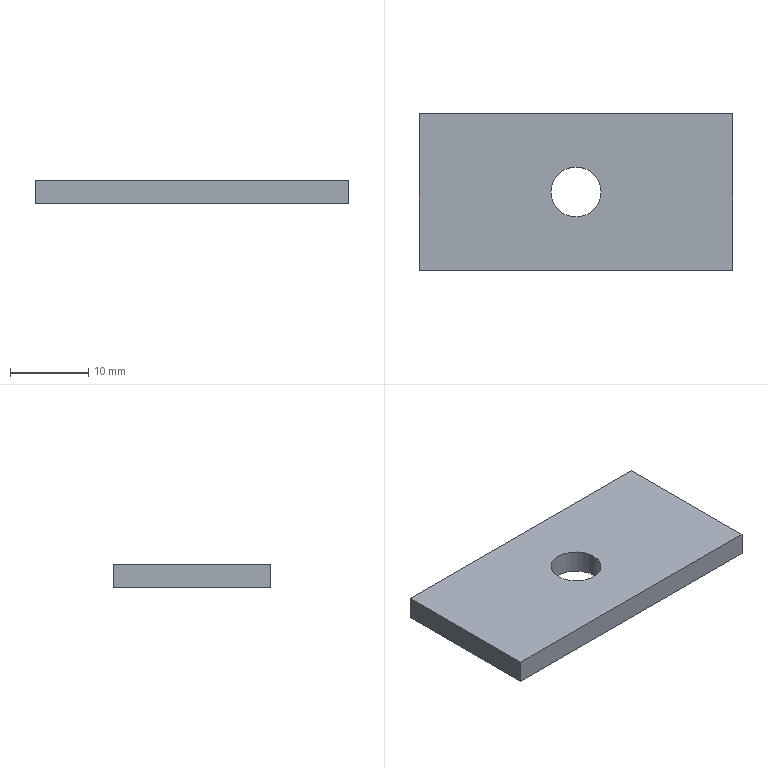Part | SolidWorks | features Extrusion 1, ICE 1 | 1 solid | 8 faces | box 40 x 20 x 3 mm | volume 2303 mm3 | plane 6 | cylinder 2 | commonest cylinder face diameters 6.4 x2
STEP:
#1=CARTESIAN_POINT('',(-3.2,0.,-1.5));
#2=VERTEX_POINT('',#1);
#3=CARTESIAN_POINT('',(3.2,0.,-1.5));
#4=VERTEX_POINT('',#3);
#5=CARTESIAN_POINT('',(0.,0.,-1.5));
#6=DIRECTION('',(0.,0.,1.));
#7=DIRECTION('',(1.,0.,0.));
#8=AXIS2_PLACEMENT_3D('',#5,#6,#7);
#9=CIRCLE('',#8,3.2);
#10=EDGE_CURVE('',#2,#4,#9,.T.);
#11=ORIENTED_EDGE('',*,*,#10,.F.);
#12=CARTESIAN_POINT('',(-3.2,0.,1.5));
#13=VERTEX_POINT('',#12);
#14=CARTESIAN_POINT('',(-3.2,0.,-11.5));
#15=DIRECTION('',(0.,0.,1.));
#16=VECTOR('',#15,1000.);
#17=LINE('',#14,#16);
#18=EDGE_CURVE('',#2,#13,#17,.T.);
#19=ORIENTED_EDGE('',*,*,#18,.T.);
#20=CARTESIAN_POINT('',(3.2,0.,1.5));
#21=VERTEX_POINT('',#20);
#22=CARTESIAN_POINT('',(0.,0.,1.5));
#23=DIRECTION('',(0.,0.,1.));
#24=DIRECTION('',(1.,0.,0.));
#25=AXIS2_PLACEMENT_3D('',#22,#23,#24);
#26=CIRCLE('',#25,3.2);
#27=EDGE_CURVE('',#13,#21,#26,.T.);
#28=ORIENTED_EDGE('',*,*,#27,.T.);
#29=CARTESIAN_POINT('',(3.2,0.,-11.5));
#30=DIRECTION('',(0.,0.,1.));
#31=VECTOR('',#30,1000.);
#32=LINE('',#29,#31);
#33=EDGE_CURVE('',#4,#21,#32,.T.);
#34=ORIENTED_EDGE('',*,*,#33,.F.);
#35=EDGE_LOOP('',(#11,#19,#28,#34));
#36=FACE_OUTER_BOUND('',#35,.T.);
#37=CARTESIAN_POINT('',(0.,0.,-11.5));
#38=DIRECTION('',(0.,0.,1.));
#39=DIRECTION('',(1.,0.,0.));
#40=AXIS2_PLACEMENT_3D('',#37,#38,#39);
#41=CYLINDRICAL_SURFACE('',#40,3.2);
#42=ADVANCED_FACE('',(#36),#41,.F.);
#43=CARTESIAN_POINT('',(-20.,10.,1.5));
#44=VERTEX_POINT('',#43);
#45=CARTESIAN_POINT('',(-20.,-10.,1.5));
#46=VERTEX_POINT('',#45);
#47=CARTESIAN_POINT('',(-20.,10.,1.5));
#48=DIRECTION('',(0.,-1.,0.));
#49=VECTOR('',#48,1000.);
#50=LINE('',#47,#49);
#51=EDGE_CURVE('',#44,#46,#50,.T.);
#52=ORIENTED_EDGE('',*,*,#51,.F.);
#53=CARTESIAN_POINT('',(-20.,10.,-1.5));
#54=VERTEX_POINT('',#53);
#55=CARTESIAN_POINT('',(-20.,10.,-1.5));
#56=DIRECTION('',(0.,0.,1.));
#57=VECTOR('',#56,1000.);
#58=LINE('',#55,#57);
#59=EDGE_CURVE('',#54,#44,#58,.T.);
#60=ORIENTED_EDGE('',*,*,#59,.F.);
#61=CARTESIAN_POINT('',(-20.,-10.,-1.5));
#62=VERTEX_POINT('',#61);
#63=CARTESIAN_POINT('',(-20.,10.,-1.5));
#64=DIRECTION('',(0.,-1.,0.));
#65=VECTOR('',#64,1000.);
#66=LINE('',#63,#65);
#67=EDGE_CURVE('',#54,#62,#66,.T.);
#68=ORIENTED_EDGE('',*,*,#67,.T.);
#69=CARTESIAN_POINT('',(-20.,-10.,-1.5));
#70=DIRECTION('',(0.,0.,1.));
#71=VECTOR('',#70,1000.);
#72=LINE('',#69,#71);
#73=EDGE_CURVE('',#62,#46,#72,.T.);
#74=ORIENTED_EDGE('',*,*,#73,.T.);
#75=EDGE_LOOP('',(#52,#60,#68,#74));
#76=FACE_OUTER_BOUND('',#75,.T.);
#77=CARTESIAN_POINT('',(-20.,10.,-1.5));
#78=DIRECTION('',(-1.,0.,0.));
#79=DIRECTION('',(0.,0.,1.));
#80=AXIS2_PLACEMENT_3D('',#77,#78,#79);
#81=PLANE('',#80);
#82=ADVANCED_FACE('',(#76),#81,.T.);
#83=CARTESIAN_POINT('',(20.,10.,1.5));
#84=VERTEX_POINT('',#83);
#85=CARTESIAN_POINT('',(20.,10.,1.5));
#86=DIRECTION('',(-1.,0.,0.));
#87=VECTOR('',#86,1000.);
#88=LINE('',#85,#87);
#89=EDGE_CURVE('',#84,#44,#88,.T.);
#90=ORIENTED_EDGE('',*,*,#89,.F.);
#91=CARTESIAN_POINT('',(20.,10.,-1.5));
#92=VERTEX_POINT('',#91);
#93=CARTESIAN_POINT('',(20.,10.,-1.5));
#94=DIRECTION('',(0.,0.,1.));
#95=VECTOR('',#94,1000.);
#96=LINE('',#93,#95);
#97=EDGE_CURVE('',#92,#84,#96,.T.);
#98=ORIENTED_EDGE('',*,*,#97,.F.);
#99=CARTESIAN_POINT('',(20.,10.,-1.5));
#100=DIRECTION('',(-1.,0.,0.));
#101=VECTOR('',#100,1000.);
#102=LINE('',#99,#101);
#103=EDGE_CURVE('',#92,#54,#102,.T.);
#104=ORIENTED_EDGE('',*,*,#103,.T.);
#105=ORIENTED_EDGE('',*,*,#59,.T.);
#106=EDGE_LOOP('',(#90,#98,#104,#105));
#107=FACE_OUTER_BOUND('',#106,.T.);
#108=CARTESIAN_POINT('',(20.,10.,-1.5));
#109=DIRECTION('',(0.,1.,0.));
#110=DIRECTION('',(0.,0.,1.));
#111=AXIS2_PLACEMENT_3D('',#108,#109,#110);
#112=PLANE('',#111);
#113=ADVANCED_FACE('',(#107),#112,.T.);
#114=CARTESIAN_POINT('',(20.,-10.,1.5));
#115=VERTEX_POINT('',#114);
#116=CARTESIAN_POINT('',(20.,-10.,1.5));
#117=DIRECTION('',(0.,1.,0.));
#118=VECTOR('',#117,1000.);
#119=LINE('',#116,#118);
#120=EDGE_CURVE('',#115,#84,#119,.T.);
#121=ORIENTED_EDGE('',*,*,#120,.F.);
#122=CARTESIAN_POINT('',(20.,-10.,-1.5));
#123=VERTEX_POINT('',#122);
#124=CARTESIAN_POINT('',(20.,-10.,-1.5));
#125=DIRECTION('',(0.,0.,1.));
#126=VECTOR('',#125,1000.);
#127=LINE('',#124,#126);
#128=EDGE_CURVE('',#123,#115,#127,.T.);
#129=ORIENTED_EDGE('',*,*,#128,.F.);
#130=CARTESIAN_POINT('',(20.,-10.,-1.5));
#131=DIRECTION('',(0.,1.,0.));
#132=VECTOR('',#131,1000.);
#133=LINE('',#130,#132);
#134=EDGE_CURVE('',#123,#92,#133,.T.);
#135=ORIENTED_EDGE('',*,*,#134,.T.);
#136=ORIENTED_EDGE('',*,*,#97,.T.);
#137=EDGE_LOOP('',(#121,#129,#135,#136));
#138=FACE_OUTER_BOUND('',#137,.T.);
#139=CARTESIAN_POINT('',(20.,-10.,-1.5));
#140=DIRECTION('',(1.,0.,0.));
#141=DIRECTION('',(0.,0.,-1.));
#142=AXIS2_PLACEMENT_3D('',#139,#140,#141);
#143=PLANE('',#142);
#144=ADVANCED_FACE('',(#138),#143,.T.);
#145=CARTESIAN_POINT('',(-20.,-10.,1.5));
#146=DIRECTION('',(1.,0.,0.));
#147=VECTOR('',#146,1000.);
#148=LINE('',#145,#147);
#149=EDGE_CURVE('',#46,#115,#148,.T.);
#150=ORIENTED_EDGE('',*,*,#149,.F.);
#151=ORIENTED_EDGE('',*,*,#73,.F.);
#152=CARTESIAN_POINT('',(-20.,-10.,-1.5));
#153=DIRECTION('',(1.,0.,0.));
#154=VECTOR('',#153,1000.);
#155=LINE('',#152,#154);
#156=EDGE_CURVE('',#62,#123,#155,.T.);
#157=ORIENTED_EDGE('',*,*,#156,.T.);
#158=ORIENTED_EDGE('',*,*,#128,.T.);
#159=EDGE_LOOP('',(#150,#151,#157,#158));
#160=FACE_OUTER_BOUND('',#159,.T.);
#161=CARTESIAN_POINT('',(-20.,-10.,-1.5));
#162=DIRECTION('',(0.,-1.,0.));
#163=DIRECTION('',(0.,0.,-1.));
#164=AXIS2_PLACEMENT_3D('',#161,#162,#163);
#165=PLANE('',#164);
#166=ADVANCED_FACE('',(#160),#165,.T.);
#167=CARTESIAN_POINT('',(0.,0.,-1.5));
#168=DIRECTION('',(0.,0.,1.));
#169=DIRECTION('',(1.,0.,0.));
#170=AXIS2_PLACEMENT_3D('',#167,#168,#169);
#171=CIRCLE('',#170,3.2);
#172=EDGE_CURVE('',#4,#2,#171,.T.);
#173=ORIENTED_EDGE('',*,*,#172,.T.);
#174=ORIENTED_EDGE('',*,*,#10,.T.);
#175=EDGE_LOOP('',(#173,#174));
#176=FACE_BOUND('',#175,.T.);
#177=ORIENTED_EDGE('',*,*,#67,.F.);
#178=ORIENTED_EDGE('',*,*,#103,.F.);
#179=ORIENTED_EDGE('',*,*,#134,.F.);
#180=ORIENTED_EDGE('',*,*,#156,.F.);
#181=EDGE_LOOP('',(#177,#178,#179,#180));
#182=FACE_OUTER_BOUND('',#181,.T.);
#183=CARTESIAN_POINT('',(0.,0.,-1.5));
#184=DIRECTION('',(0.,0.,1.));
#185=DIRECTION('',(1.,0.,0.));
#186=AXIS2_PLACEMENT_3D('',#183,#184,#185);
#187=PLANE('',#186);
#188=ADVANCED_FACE('',(#176,#182),#187,.F.);
#189=CARTESIAN_POINT('',(0.,0.,1.5));
#190=DIRECTION('',(0.,0.,1.));
#191=DIRECTION('',(1.,0.,0.));
#192=AXIS2_PLACEMENT_3D('',#189,#190,#191);
#193=CIRCLE('',#192,3.2);
#194=EDGE_CURVE('',#21,#13,#193,.T.);
#195=ORIENTED_EDGE('',*,*,#194,.F.);
#196=ORIENTED_EDGE('',*,*,#27,.F.);
#197=EDGE_LOOP('',(#195,#196));
#198=FACE_BOUND('',#197,.T.);
#199=ORIENTED_EDGE('',*,*,#51,.T.);
#200=ORIENTED_EDGE('',*,*,#149,.T.);
#201=ORIENTED_EDGE('',*,*,#120,.T.);
#202=ORIENTED_EDGE('',*,*,#89,.T.);
#203=EDGE_LOOP('',(#199,#200,#201,#202));
#204=FACE_OUTER_BOUND('',#203,.T.);
#205=CARTESIAN_POINT('',(0.,0.,1.5));
#206=DIRECTION('',(0.,0.,1.));
#207=DIRECTION('',(1.,0.,0.));
#208=AXIS2_PLACEMENT_3D('',#205,#206,#207);
#209=PLANE('',#208);
#210=ADVANCED_FACE('',(#198,#204),#209,.T.);
#211=ORIENTED_EDGE('',*,*,#18,.F.);
#212=ORIENTED_EDGE('',*,*,#172,.F.);
#213=ORIENTED_EDGE('',*,*,#33,.T.);
#214=ORIENTED_EDGE('',*,*,#194,.T.);
#215=EDGE_LOOP('',(#211,#212,#213,#214));
#216=FACE_OUTER_BOUND('',#215,.T.);
#217=CARTESIAN_POINT('',(0.,0.,-11.5));
#218=DIRECTION('',(0.,0.,1.));
#219=DIRECTION('',(1.,0.,0.));
#220=AXIS2_PLACEMENT_3D('',#217,#218,#219);
#221=CYLINDRICAL_SURFACE('',#220,3.2);
#222=ADVANCED_FACE('',(#216),#221,.F.);
#223=CLOSED_SHELL('',(#42,#82,#113,#144,#166,#188,#210,#222));
#224=MANIFOLD_SOLID_BREP('',#223);
#225=CARTESIAN_POINT('',(0.,0.,0.));
#226=DIRECTION('',(0.,0.,1.));
#227=DIRECTION('',(1.,0.,0.));
#228=AXIS2_PLACEMENT_3D('',#225,#226,#227);
#229=(LENGTH_UNIT()NAMED_UNIT(*)SI_UNIT(.MILLI.,.METRE.));
#230=UNCERTAINTY_MEASURE_WITH_UNIT(LENGTH_MEASURE(0.00001),#229,'','');
#231=(NAMED_UNIT(*)PLANE_ANGLE_UNIT()SI_UNIT($,.RADIAN.));
#232=(NAMED_UNIT(*)SI_UNIT($,.STERADIAN.)SOLID_ANGLE_UNIT());
#233=(GEOMETRIC_REPRESENTATION_CONTEXT(3)GLOBAL_UNCERTAINTY_ASSIGNED_CONTEXT((#230))GLOBAL_UNIT_ASSIGNED_CONTEXT((#229,#231,#232))REPRESENTATION_CONTEXT('',''));
#234=ADVANCED_BREP_SHAPE_REPRESENTATION('',(#224,#228),#233);